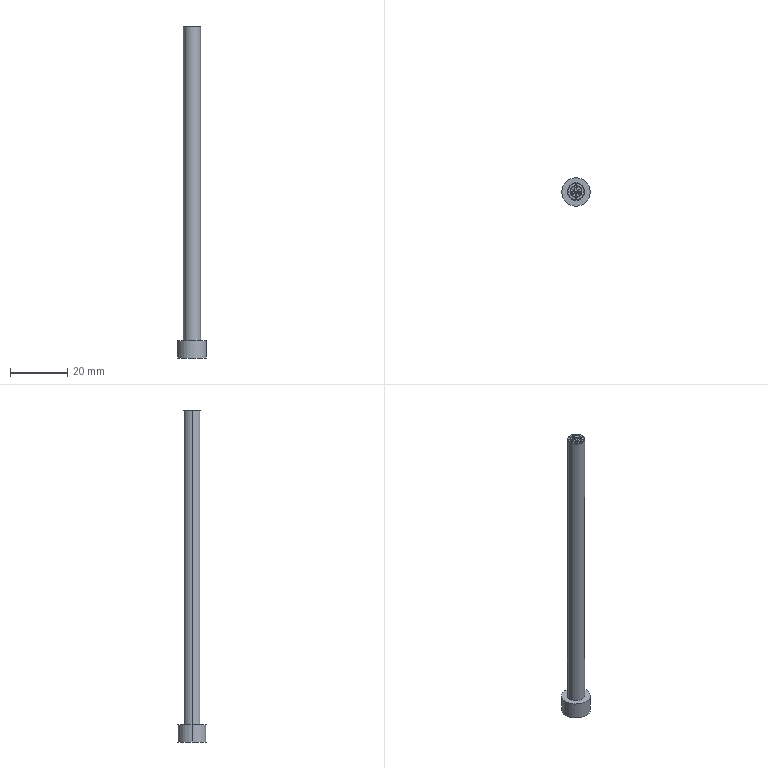Part | SolidWorks | features BaseBody 1 | 1 solid | 129 faces | box 10 x 10 x 116.348 mm | volume 3590 mm3 | plane 81 | cylinder 32 | spline 16 | commonest cylinder face diameters 4.15 x12 5.7 x12 3.85 x4 6 x2 10 x2